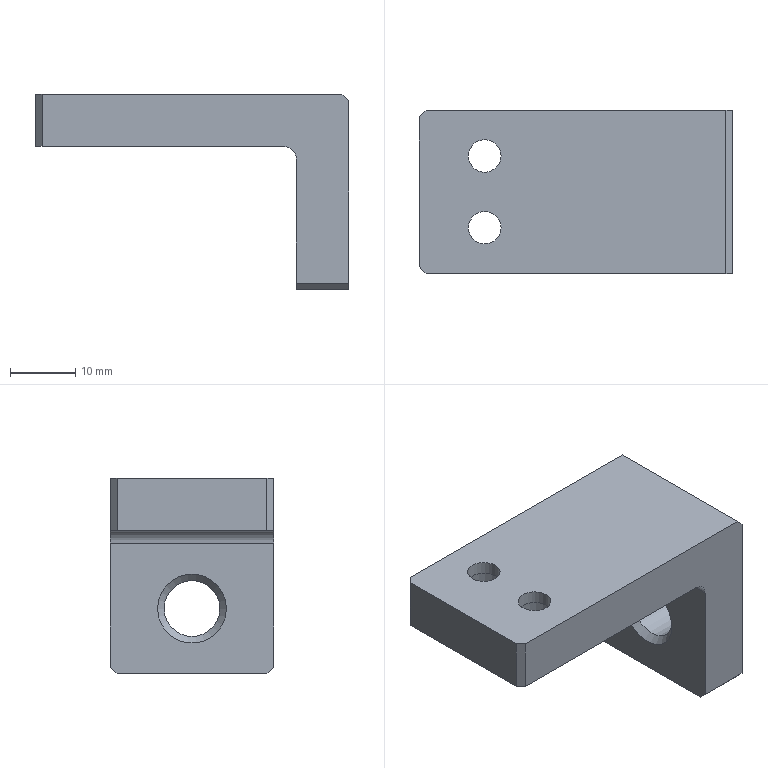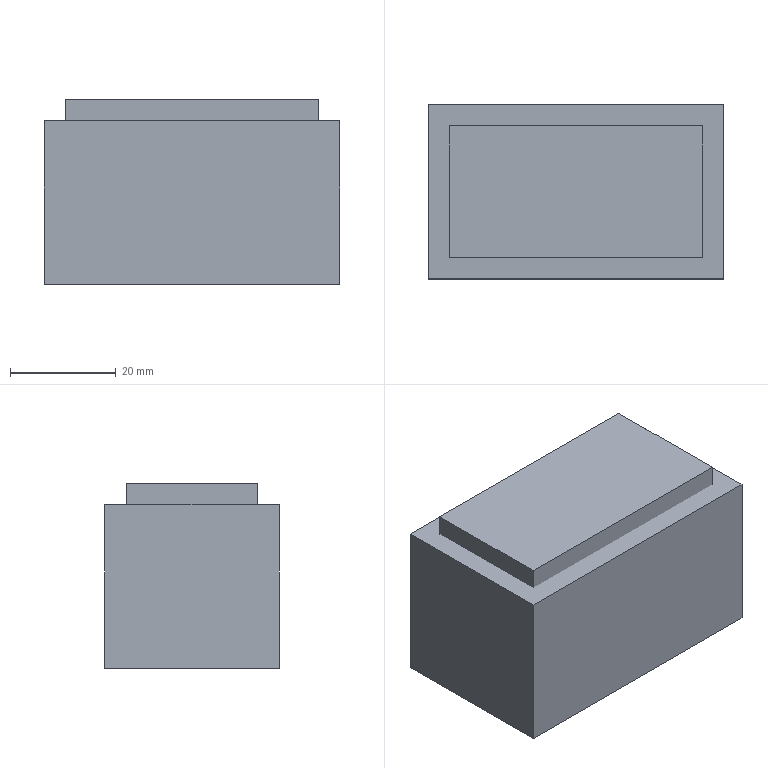CAM job | NX | 3+2 milling, drilling | part box 48 x 25 x 30 mm | stock box 56 x 33 x 35 mm
Tools:
number,name,description,diameter,corner_radius,flute_length,length,flutes
1,D63,Milling Tool-5 Parameters,63.0,0.0,50.0,75.0,2
2,D10,Milling Tool-5 Parameters,10.0,0.0,50.0,75.0,2
9,D6A45,Milling Tool-5 Parameters,6.0,0.0,3.0,3.0,2
14,5.0ZT,Drilling Tool,4.5,0.0,35.0,50.0,2
4,D6,Milling Tool-5 Parameters,6.0,0.0,50.0,75.0,2
Operations:
program,operation,operation_type,tool,method,geometry_group,spindle_rpm,surface_speed,feed_per_tooth,feed_cut,feed_plunge,cut_length_mm,path_length_mm,cut_time_min,machine_time_min
1-55-35-30毛胚,FLOOR_WALL,VolumeBased25DMillingOperation,D63,METHOD,A,6500.0,0.0,0.0,1250.0,100.0,131.0,185.0,0.1048,0.1102
1-55-35-30毛胚,ADAPTIVE_MILLING,CavityMilling,D10,METHOD,A,7000.0,219.0,0.1429,2000.0,1000.0,2183.168,2389.284,1.095,1.115
1-55-35-30毛胚,ZLEVEL_PROFILE_COPY_COPY_1_COPY,ZLevelMilling,D10,METHOD,A,6500.0,326.0,0.0769,1000.0,1000.0,370.489,488.018,0.3705,0.3822
1-55-35-30毛胚,DRILLING,Operation,D6A45,METHOD,A,4000.0,75.0,0.0312,250.0,0.0,8.0,90.402,0.032,0.0402
1-55-35-30毛胚,DRILLING_COPY_1,Operation,5.0ZT,METHOD,A,2000.0,20.0,0.05,200.0,0.0,15.704,105.809,0.0785,0.0875
1-55-35-30毛胚,ZLEVEL_PROFILE_COPY_1_COPY_COPY_COPY_COPY_COPY,ZLevelMilling,D6A45,METHOD,A,7000.0,131.0,0.0714,1000.0,1000.0,172.732,384.403,0.1727,0.1939
2-55-35-30毛胚,FLOOR_WALL_COPY,VolumeBased25DMillingOperation,D63,METHOD,B,6500.0,0.0,0.0,1250.0,100.0,615.0,1333.001,0.492,0.5638
2-55-35-30毛胚,ADAPTIVE_MILLING_COPY,CavityMilling,D10,METHOD,B,7000.0,219.0,0.1429,2000.0,1000.0,2862.654,3452.3,1.439,1.498
2-55-35-30毛胚,FLOOR_WALL_1_COPY_COPY_1_COPY,VolumeBased25DMillingOperation,D10,METHOD,B,7000.0,219.0,0.0714,1000.0,1000.0,395.815,539.818,0.3958,0.4102
2-55-35-30毛胚,ZLEVEL_PROFILE_COPY_COPY_1_COPY_COPY,ZLevelMilling,D10,METHOD,B,6500.0,326.0,0.0769,1000.0,1000.0,44.076,141.076,0.0441,0.0538
2-55-35-30毛胚,ZLEVEL_PROFILE_1,ZLevelMilling,D10,METHOD,B,7000.0,131.0,0.1786,2500.0,1000.0,2423.813,2522.863,0.972,0.9819
2-55-35-30毛胚,HOLE_MILLING,CylinderMilling,D6,METHOD,B,7000.0,131.0,0.1214,1700.0,100.0,279.147,509.147,0.1642,0.1872
2-55-35-30毛胚,ZLEVEL_PROFILE_COPY_1_COPY_COPY_COPY_COPY_COPY_1,ZLevelMilling,D6A45,METHOD,B,7000.0,131.0,0.0714,1000.0,1000.0,74.036,137.036,0.074,0.0803
2-55-35-30毛胚,ZLEVEL_PROFILE_COPY_1_COPY_COPY_COPY_COPY_COPY_1_COPY,ZLevelMilling,D6A45,METHOD,B,7000.0,131.0,0.0714,1000.0,1000.0,154.057,512.709,0.1541,0.1899
3-55-35-30毛胚,HOLE_MILLING_COPY,CylinderMilling,D6,METHOD,C,7000.0,131.0,0.1214,1700.0,100.0,183.606,251.106,0.108,0.1148
3-55-35-30毛胚,ZLEVEL_PROFILE_COPY_1_COPY_COPY_COPY_COPY_COPY_1_COPY_1,ZLevelMilling,D6A45,METHOD,C,7000.0,131.0,0.0714,1000.0,1000.0,141.268,282.959,0.1413,0.1554